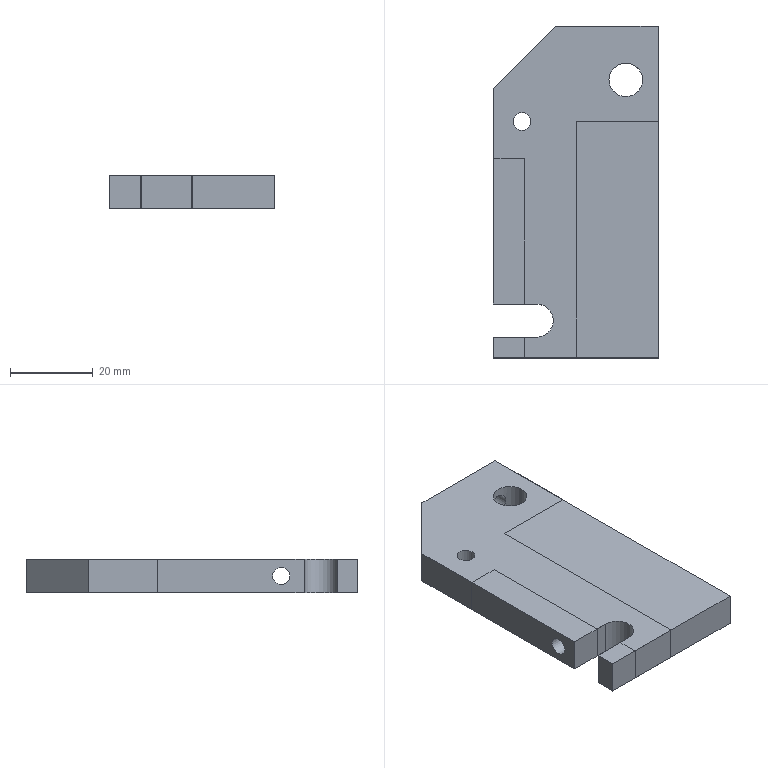NC program | NX | posted with a generic post | part box 40 x 80 x 8 mm
Whole program:
N10 G17 G21 G94 G90
(ADAPTIVE_MILLING , TOOL : D10-30-D10-75-3T-ROUGH)
N12 T01 M6
N14 G54
N16 G17 G0 G90 X-0.719 Y33.082 S3000 M3
N18 G43 Z20. H1
N20 Z3.1
N22 G94 G1 X-0.716 Y32.932 Z2.163 F1500.
N24 X-0.713 Y32.782 Z1.792
N26 X-0.71 Y32.632 Z1.52
N28 X-0.707 Y32.482 Z1.3
N30 X-0.704 Y32.332 Z1.116
N32 X-0.701 Y32.182 Z0.958
N34 X-0.698 Y32.032 Z0.82
N36 X-0.695 Y31.882 Z0.7
N38 X-0.692 Y31.732 Z0.595
N40 X-0.688 Y31.582 Z0.502
N42 X-0.685 Y31.432 Z0.421
N44 X-0.682 Y31.282 Z0.35
N46 X-0.679 Y31.132 Z0.29
N48 X-0.676 Y30.982 Z0.238
N50 X-0.673 Y30.832 Z0.195
N52 X-0.67 Y30.682 Z0.161
N54 X-0.667 Y30.532 Z0.134
N56 X-0.664 Y30.382 Z0.115
N58 X-0.661 Y30.232 Z0.104
N60 X-0.658 Y30.082 Z0.1
N62 X-0.624 Y28.462
N64 G3 X0.024 Y27.54 R1.011
N66 X2.218 Y27.216 R8.479
N68 X11.422 Y27.1 R194.322
N70 G1 X39.422 Y27.099
N72 G2 X44.024 Y24.676 R5.712
N74 X45.709 Y20.39 R9.765
N76 X46.075 Y14.707 R38.659
N78 G1 X46.098 Y7.207
N80 X46.096 Y-20.46
N82 G2 X43.644 Y-25.047 R5.72
N84 X39.252 Y-26.733 R9.919
N86 X33.467 Y-27.079 R41.286
N88 G1 X26.218 Y-27.1
N90 X-39.462 Y-27.097
N92 G2 X-44.048 Y-24.645 R5.719
N94 X-45.734 Y-20.252 R9.931
N96 X-46.08 Y-14.467 R41.275
N98 G1 X-46.101 Y-7.217
N100 X-46.099 Y20.46
N102 G2 X-43.646 Y25.047 R5.719
N104 X-39.253 Y26.732 R9.931
N106 X-33.469 Y27.079 R41.275
N108 G1 X-26.219 Y27.1
N110 X-2.119 Y27.097
N112 G2 X2.81 Y26.809 R819.319
N114 G3 X12.522 Y26.701 R286.424
N116 G1 X37.722 Y26.699
N118 G2 X43.64 Y23.314 R7.101
N120 X45.299 Y18.58 R11.962
N122 X45.672 Y12.446 R45.859
N124 G1 X45.698 Y4.546
N126 X45.697 Y-18.722
N128 G2 X42.35 Y-24.615 R7.089
N130 X37.576 Y-26.3 R11.916
N132 X31.642 Y-26.671 R44.728
N134 G1 X23.692 Y-26.699
N136 X-37.723 Y-26.698
N138 G2 X-43.617 Y-23.349 R7.088
N140 X-45.301 Y-18.575 R11.921
N142 X-45.678 Y-12.191 R47.36
N144 G1 X-45.7 Y-5.941
N146 Y18.622
N148 G2 X-42.35 Y24.616 R7.087
N150 X-37.576 Y26.3 R11.921
N152 X-31.193 Y26.677 R47.36
N154 G1 X-24.943 Y26.699
N156 X-3.73 Y26.698
N158 G2 X2.84 Y26.421 R237.984
N160 G3 X13.622 Y26.301 R334.657
N162 G1 X35.972 Y26.3
N164 G2 X43.459 Y21.85 R8.144
N166 X44.965 Y16.642 R14.601
N168 X45.282 Y9.653 R64.652
N170 G1 X45.298 Y3.003
N172 X45.297 Y-17.047
N174 G2 X40.938 Y-24.409 R8.12
N176 X35.89 Y-25.934 R14.195
N178 X29.303 Y-26.277 R56.959
N180 G1 X21.453 Y-26.299
N182 X-36.047 Y-26.298
N184 G2 X-43.413 Y-21.934 R8.118
N186 X-44.935 Y-16.889 R14.217
N188 X-45.279 Y-10.252 R57.3
N190 G1 X-45.3 Y-2.552
N192 X-45.299 Y17.048
N194 G2 X-40.936 Y24.412 R8.118
N196 X-35.89 Y25.934 R14.218
N198 X-29.253 Y26.277 R57.3
N200 G1 X-21.553 Y26.299
N202 X-4.979 Y26.298
N204 G2 X2.923 Y26.026 R253.671
N206 G3 X15.222 Y25.901 R401.917
N208 G1 X34.472 Y25.9
N210 G2 X38.99 Y24.999 R9.989
N212 X43.369 Y20.219 R9.282
N214 X44.633 Y14.737 R18.014
N216 X44.889 Y6.893 R93.499
N218 G1 X44.897 Y1.943
N220 Y-15.472
N222 G2 X43.996 Y-19.99 R9.988
N224 X39.156 Y-24.396 R9.305
N226 X33.568 Y-25.65 R18.418
N228 X25.924 Y-25.89 R96.511
N230 G1 X20.974 Y-25.899
N232 X-34.473 Y-25.898
N234 G2 X-38.991 Y-24.997 R9.99
N236 X-43.369 Y-20.219 R9.282
N238 X-44.635 Y-14.737 R18.005
N240 X-44.891 Y-6.994 R92.212
N242 G1 X-44.9 Y-0.944
N244 X-44.899 Y15.472
N246 G2 X-43.998 Y19.99 R9.989
N248 X-39.221 Y24.368 R9.282
N250 X-33.738 Y25.634 R18.005
N252 X-25.995 Y25.89 R92.222
N254 G1 X-19.945 Y25.899
N256 X-6.179 Y25.898
N258 G2 X3.109 Y25.627 R288.66
N260 G3 X15.272 Y25.501 R440.021
N262 G1 X33.222 Y25.499
N264 G2 X37.685 Y24.777 R11.809
N266 X42.744 Y19.814 R9.555
N268 X44.158 Y14.317 R17.56
N270 X44.48 Y6.828 R75.391
N272 G1 X44.497 Y-0.372
N274 X44.496 Y-14.122
N276 G2 X43.864 Y-18.451 R12.256
N278 X38.889 Y-23.708 R9.502
N280 X33.202 Y-25.171 R17.61
N282 X25.462 Y-25.484 R79.927
N284 G1 X18.862 Y-25.498
N286 X-33.123
N288 G2 X-37.453 Y-24.865 R12.256
N290 X-42.708 Y-19.891 R9.504
N292 X-44.161 Y-14.304 R17.449
N294 X-44.484 Y-6.614 R76.99
N296 G1 X-44.499 Y-0.564
N298 Y14.122
N300 G2 X-43.866 Y18.452 R12.255
N302 X-38.892 Y23.707 R9.504
N304 X-33.305 Y25.16 R17.45
N306 X-25.615 Y25.483 R76.991
N308 G1 X-19.565 Y25.498
N310 X-7.279
N312 G2 X3.101 Y25.232 R315.659
N314 G3 X15.572 Y25.102 R473.15
N316 G1 X31.922 Y25.1
N318 G2 X36.321 Y24.557 R14.429
N320 X42.155 Y19.383 R9.828
N322 X43.719 Y13.621 R17.669
N324 X44.08 Y5.583 R75.857
N326 G1 X44.097 Y-2.117
N328 G2 X44.075 Y-14.022 R854.441
N330 X42.651 Y-19.324 R10.75
N332 X37.33 Y-23.618 R10.507
N334 X31.526 Y-24.834 R21.057
N336 X23.432 Y-25.088 R104.823
N338 G1 X16.832 Y-25.098
N340 X-31.873 Y-25.097
N342 G2 X-36.178 Y-24.598 R14.783
N344 X-42.154 Y-19.384 R9.816
N346 X-43.702 Y-13.771 R17.466
N348 X-44.079 Y-5.985 R70.636
N350 G1 X-44.099 Y0.665
N352 G2 X-44.077 Y14.021 R944.397
N354 X-42.652 Y19.326 R10.747
N356 X-37.473 Y23.562 R10.454
N358 X-31.828 Y24.805 R20.302
N360 X-23.286 Y25.089 R100.222
N362 G1 X-18.336 Y25.098
N364 G2 X-3.43 Y25.04 R736.675
N366 G3 X16.822 Y24.702 R491.196
N368 G1 X30.672 Y24.7
N370 G2 X35.088 Y24.271 R17.569
N372 X41.664 Y18.796 R10.156
N374 X43.286 Y12.942 R18.042
N376 X43.67 Y5.356 R69.858
N378 G1 X43.696 Y-1.794
N380 G2 X43.664 Y-13.221 R565.835
N382 X42.301 Y-18.495 R11.448
N384 X36.974 Y-23.04 R10.705
N386 X31.047 Y-24.387 R20.607
N388 X22.655 Y-24.686 R96.522
N390 G1 X16.055 Y-24.698
N392 X-30.673 Y-24.697
N394 G2 X-35.138 Y-24.256 R17.414
N396 X-41.664 Y-18.798 R10.155
N398 X-43.287 Y-12.943 R18.041
N400 X-43.673 Y-5.307 R69.917
N402 G1 X-43.699 Y1.843
N404 G2 X-43.667 Y13.221 R562.693
N406 X-42.229 Y18.624 R11.384
N408 X-36.884 Y23.077 R10.77
N410 X-31.05 Y24.386 R20.792
N412 X-22.658 Y24.686 R96.37
N414 G1 X-17.158 Y24.698
N416 G2 X-2.78 Y24.616 R565.256
N418 G3 X17.222 Y24.302 R497.288
N420 G1 X29.422 Y24.301
N422 G2 X33.949 Y23.949 R21.442
N424 X41.202 Y18.191 R10.484
N426 X42.861 Y12.245 R18.494
N428 X43.267 Y4.51 R69.668
N430 X43.271 Y-12.072 R903.237
N432 X42.184 Y-17.22 R12.904
N434 X36.655 Y-22.454 R10.785
N436 X30.707 Y-23.927 R20.022
N438 X22.318 Y-24.28 R85.309
N440 G1 X14.618 Y-24.298
N442 X-29.473 Y-24.297
N444 G2 X-34.048 Y-23.924 R20.815
N446 X-41.198 Y-18.199 R10.48
N448 X-42.856 Y-12.295 R18.441
N450 X-43.27 Y-4.46 R69.348
N452 X-43.273 Y12.072 R903.184
N454 X-42.187 Y17.22 R12.901
N456 X-36.649 Y22.457 R10.788
N458 X-30.651 Y23.933 R20.145
N460 X-22.311 Y24.28 R86.022
N462 X-3.762 Y24.234 R842.135
N464 G3 X16.972 Y23.902 R589.615
N466 G2 X30.272 Y23.87 R817.304
N468 X35.433 Y22.825 R13.687
N470 X40.947 Y17.183 R11.01
N472 X42.497 Y11.103 R20.146
N474 X42.877 Y2.565 R83.861
N476 X42.865 Y-11.271 R673.681
N478 X41.821 Y-16.433 R13.68
N480 X36.181 Y-21.947 R11.008
N482 X30.101 Y-23.498 R20.156
N484 X22.063 Y-23.873 R79.7
N486 G1 X13.763 Y-23.897
N488 X-28.273
N490 G2 X-33.005 Y-23.579 R24.995
N492 X-40.778 Y-17.537 R10.798
N494 X-42.444 Y-11.542 R19.054
N496 X-42.872 Y-3.308 R72.694
N498 X-42.868 Y11.272 R673.669
N500 X-41.823 Y16.433 R13.677
N502 X-36.131 Y21.969 R11.023
N504 X-30.047 Y23.504 R20.331
N506 X-21.759 Y23.876 R82.622
N508 X-2.86 Y23.807 R680.934
N510 G3 X18.222 Y23.502 R579.313
N512 G2 X29.521 Y23.465 R553.103
N514 X34.784 Y22.41 R14.313
N516 X40.507 Y16.586 R11.272
N518 X42.077 Y10.458 R20.555
N520 X42.469 Y2.372 R79.047
N522 X42.459 Y-10.528 R490.91
N524 X41.424 Y-15.744 R14.313
N526 X35.702 Y-21.453 R11.233
N528 X29.635 Y-23.057 R20.14
N530 X21.15 Y-23.472 R78.544
N532 G1 X12.9 Y-23.497
N534 X-27.223
N536 G2 X-32.059 Y-23.212 R28.734
N538 X-40.389 Y-16.838 R11.113
N540 X-42.057 Y-10.635 R19.958
N542 X-42.468 Y-2.599 R75.097
N544 X-42.466 Y10.422 R554.767
N546 X-41.505 Y15.554 R14.678
N548 X-35.704 Y21.452 R11.207
N550 X-29.438 Y23.08 R20.455
N552 X-21.051 Y23.473 R81.406
N554 X4.464 Y23.214 R604.269
N556 G3 X25.422 Y23.102 R966.669
N558 G2 X30.615 Y22.917 R44.386
N560 X37.603 Y19.646 R11.532
N562 X40.882 Y13.796 R13.568
N564 X41.902 Y7.037 R30.903
N566 X42.094 Y-4.26 R214.857
N568 X42.002 Y-10.708 R100.555
N570 X40.299 Y-16.505 R12.789
N572 X34.425 Y-21.32 R11.94
N574 X28.049 Y-22.746 R23.095
N576 X19.108 Y-23.081 R101.832
N578 G1 X11.959 Y-23.097
N580 X-26.673 Y-23.095
N582 G2 X-31.703 Y-22.741 R26.76
N584 X-39.936 Y-16.294 R11.35
N586 X-41.634 Y-10.045 R20.219
N588 X-42.068 Y-1.711 R75.709
N590 X-42.05 Y9.939 R336.332
N592 X-40.915 Y15.336 R14.486
N594 X-35.093 Y21.03 R11.506
N596 X-28.874 Y22.654 R20.788
N598 X-20.638 Y23.067 R78.035
N600 X4.214 Y22.821 R594.688
N602 G3 X25.422 Y22.701 R984.655
N604 G2 X30.559 Y22.421 R33.455
N606 X39.529 Y15.671 R11.636
N608 X41.223 Y9.372 R20.737
N610 X41.664 Y0.887 R77.377
N612 X41.644 Y-9.212 R261.519
N614 X40.525 Y-14.666 R15.127
N616 X34.54 Y-20.59 R11.713
N618 X28.127 Y-22.254 R21.272
N620 X19.542 Y-22.669 R82.502
N622 G1 X11.792 Y-22.696
N624 X-25.523
N626 G2 X-30.757 Y-22.384 R31.453
N628 X-39.528 Y-15.672 R11.618
N630 X-41.224 Y-9.374 R20.756
N632 X-41.668 Y-0.739 R78.339
N634 X-41.644 Y9.26 R252.258
N636 X-40.528 Y14.664 R15.037
N638 X-34.536 Y20.591 R11.713
N640 X-28.169 Y22.248 R21.245
N642 X-19.383 Y22.671 R83.267
N644 X3.964 Y22.428 R587.164
N646 G3 X25.172 Y22.298 R993.4
N648 G2 X30.45 Y21.916 R28.573
N650 X39.063 Y15.188 R11.812
N652 X40.81 Y8.749 R21.011
N654 X41.264 Y0.016 R79.088
N656 X41.233 Y-8.633 R189.322
N658 X40.065 Y-14.178 R15.34
N660 X33.936 Y-20.181 R11.943
N662 X27.52 Y-21.839 R21.672
N664 X18.735 Y-22.269 R83.286
N666 G1 X9.935 Y-22.296
N668 X-24.573 Y-22.295
N670 G2 X-29.959 Y-22. R34.738
N672 X-39.095 Y-15.122 R11.851
N674 X-40.814 Y-8.726 R21.164
N676 X-41.263 Y-0.292 R77.052
N678 X-41.231 Y8.707 R186.101
N680 X-40.035 Y14.249 R15.159
N682 X-33.986 Y20.157 R11.94
N684 X-27.622 Y21.826 R21.522
N686 X-18.988 Y22.266 R80.32
N688 X3.416 Y22.041 R556.79
N690 G3 X24.422 Y21.898 R946.655
N692 G2 X29.702 Y21.531 R30.293
N694 X38.634 Y14.644 R12.023
N696 X40.369 Y8.355 R21.059
N698 X40.852 Y0.024 R72.506
N700 X40.81 Y-8.274 R136.124
N702 X39.518 Y-13.892 R15.097
N704 X33.372 Y-19.76 R12.174
N706 X26.908 Y-21.427 R22.054
N708 X18.473 Y-21.861 R80.674
N710 G1 X9.073 Y-21.896
N712 X-23.573 Y-21.895
N714 G2 X-29.012 Y-21.64 R40.091
N716 X-36.049 Y-18.319 R12.222
N718 X-39.538 Y-12.298 R14.066
N720 X-40.667 Y-5.303 R31.062
N722 X-40.823 Y8.092 R160.177
N724 X-39.617 Y13.68 R15.53
N726 X-33.449 Y19.724 R12.121
N728 X-27.042 Y21.41 R21.8
N730 X-18.209 Y21.865 R81.15
N732 X4.227 Y21.625 R606.053
N734 G3 X23.972 Y21.495 R949.588
N736 G2 X29.396 Y21.064 R28.549
N738 X38.163 Y14.199 R12.184
N740 X39.949 Y7.821 R21.194
N742 X40.446 Y-0.409 R71.049
N744 X40.391 Y-7.807 R102.754
N746 X38.996 Y-13.551 R15.059
N748 X32.883 Y-19.311 R12.36
N750 X26.275 Y-21.021 R22.401
N752 X17.691 Y-21.461 R82.28
N754 G1 X8.291 Y-21.496
N756 X-22.659 Y-21.495
N758 G2 X-28.349 Y-21.239 R43.043
N760 X-35.311 Y-18.105 R12.542
N762 X-39.015 Y-12.066 R13.938
N764 X-40.228 Y-5.138 R29.621
N766 X-40.41 Y7.555 R130.078
N768 X-39.15 Y13.233 R15.667
N770 X-32.885 Y19.309 R12.324
N772 X-26.279 Y21.019 R22.415
N774 X-17.295 Y21.466 R84.914
N776 X3.213 Y21.247 R558.526
N778 G3 X23.473 Y21.092 R982.573
N780 G2 X28.944 Y20.626 R27.902
N782 X37.781 Y13.578 R12.376
N784 X39.557 Y7.094 R21.817
N786 X40.053 Y-1.637 R76.269
N788 X39.911 Y-8.032 R59.227
N790 X37.852 Y-14.287 R13.739
N792 X31.789 Y-19.13 R12.961
N794 X25.186 Y-20.669 R24.327
N796 X16.049 Y-21.07 R96.113
N798 G1 X7.249 Y-21.095
N800 X-21.801
N802 G2 X-27.592 Y-20.852 R46.657
N804 X-34.274 Y-18.134 R13.003
N806 X-38.408 Y-12.066 R13.591
N808 X-39.76 Y-5.268 R27.304
N810 X-40.001 Y6.923 R109.018
N812 X-38.747 Y12.654 R16.047
N814 X-32.387 Y18.869 R12.481
N816 X-25.737 Y20.603 R22.617
N818 X-16.903 Y21.061 R82.904
N820 X3.857 Y20.835 R587.071
N822 G3 X22.824 Y20.691 R971.585
N824 G2 X28.394 Y20.211 R28.452
N826 X37.342 Y13.087 R12.536
N828 X39.15 Y6.5 R22.085
N830 X39.65 Y-2.481 R76.95
N832 X39.376 Y-8.418 R38.219
N834 X35.884 Y-15.687 R12.754
N836 X29.751 Y-19.248 R14.592
N838 X22.713 Y-20.43 R31.386
N840 X11.869 Y-20.689 R169.176
N842 G1 X6.369 Y-20.695
N844 X-21.481 Y-20.693
N846 G2 X-27.22 Y-20.414 R42.746
N848 X-34.142 Y-17.395 R13.009
N850 X-38.118 Y-11.155 R14.099
N852 X-39.382 Y-4.338 R29.122
N854 X-39.579 Y6.504 R90.847
N856 X-38.237 Y12.317 R15.896
N858 X-31.834 Y18.459 R12.668
N860 X-25.229 Y20.185 R22.836
N862 X-16.496 Y20.655 R80.678
N864 X4.153 Y20.431 R597.167
N866 G3 X22.026 Y20.292 R917.556
N868 G2 X27.698 Y19.83 R30.306
N870 X36.943 Y12.521 R12.715
N872 X38.759 Y5.788 R22.609
N874 X39.14 Y-6.242 R72.388
N876 X37.59 Y-12.252 R15.394
N878 X31.199 Y-18.09 R12.902
N880 X24.534 Y-19.792 R23.424
N882 X15.55 Y-20.259 R84.976
N884 G1 X5.651 Y-20.295
N886 X-20.099 Y-20.294
N888 G2 X-26.192 Y-20.066 R53.835
N890 X-32.664 Y-17.74 R13.856
N892 X-37.344 Y-11.597 R13.443
N894 X-38.873 Y-4.833 R25.548
N896 X-39.141 Y6.253 R73.358
N898 X-37.608 Y12.22 R15.402
N900 X-31.255 Y18.065 R12.886
N902 X-24.645 Y19.778 R23.234
N904 X-15.513 Y20.257 R83.462
N906 X3.407 Y20.046 R571.534
N908 G3 X21.627 Y19.888 R982.087
N910 G2 X27.296 Y19.389 R29.352
N912 X36.49 Y12.08 R12.846
N914 X38.341 Y5.303 R22.69
N916 X38.711 Y-5.826 R62.165
N918 X37.006 Y-12.047 R15.207
N920 X30.672 Y-17.676 R13.094
N922 X23.96 Y-19.385 R23.746
N924 X14.677 Y-19.86 R87.473
N926 G1 X4.777 Y-19.894
N928 X-19.823 Y-19.893
N930 G2 X-26.012 Y-19.608 R47.304
N932 X-32.784 Y-16.854 R13.577
N934 X-37.133 Y-10.534 R14.038
N936 X-38.528 Y-3.642 R27.978
N938 X-38.723 Y5.697 R63.623
N940 X-37.115 Y11.848 R15.459
N942 X-30.696 Y17.664 R13.055
N944 X-23.938 Y19.387 R23.763
N946 X-14.605 Y19.858 R86.849
N948 X4.251 Y19.63 R626.009
N950 G3 X20.629 Y19.492 R875.153
N952 G2 X26.454 Y19.041 R32.844
N954 X36.072 Y11.572 R13.007
N956 X37.919 Y4.845 R22.834
N958 X38.272 Y-5.483 R53.279
N960 X36.45 Y-11.783 R14.988
N962 X30.058 Y-17.303 R13.289
N964 X23.24 Y-18.997 R24.401
N966 X14.256 Y-19.456 R88.108
N968 X3.756 Y-19.494 R739.957
N970 G1 X-19.044 Y-19.493
N972 G2 X-25.334 Y-19.218 R50.202
N974 X-31.905 Y-16.73 R14.003
N976 X-36.564 Y-10.423 R13.855
N978 X-38.094 Y-3.357 R26.939
N980 X-38.261 Y5.63 R51.941
N982 X-36.32 Y12.005 R14.723
N984 X-29.918 Y17.362 R13.387
N986 X-23.138 Y19.009 R24.81
N988 X-13.553 Y19.458 R92.085
N990 X4.249 Y19.231 R654.526
N992 G3 X20.082 Y19.091 R885.67
N994 G2 X25.956 Y18.625 R32.98
N996 X35.62 Y11.142 R13.126
N998 X37.488 Y4.469 R22.737
N1000 X37.818 Y-5.257 R45.53
N1002 X35.701 Y-11.824 R14.535
N1004 X29.308 Y-16.989 R13.613
N1006 X22.419 Y-18.622 R25.473
N1008 X12.933 Y-19.063 R96.892
N1010 G1 X3.033 Y-19.094
N1012 X-18.267 Y-19.093
N1014 G2 X-24.509 Y-18.846 R55.144
N1016 X-31.021 Y-16.586 R14.584
N1018 X-36.019 Y-10.24 R13.736
N1020 X-37.646 Y-3.196 R25.956
N1022 X-37.812 Y5.339 R44.396
N1024 X-35.637 Y11.923 R14.417
N1026 X-29.299 Y16.992 R13.641
N1028 X-22.362 Y18.627 R25.593
N1030 X-12.625 Y19.055 R96.329
N1032 X5.64 Y18.808 R830.443
N1034 G3 X19.835 Y18.686 R992.222
N1036 G2 X25.751 Y18.15 R30.641
N1038 X35.249 Y10.55 R13.258
N1040 X37.115 Y3.676 R23.421
N1042 X37.364 Y-4.953 R39.363
N1044 X35.065 Y-11.654 R14.294
N1046 X28.741 Y-16.599 R13.827
N1048 X21.801 Y-18.223 R25.939
N1050 X12.215 Y-18.664 R99.214
N1052 G1 X2.315 Y-18.693
N1054 X-17.485 Y-18.692
N1056 G2 X-23.976 Y-18.438 R57.076
N1058 X-30.502 Y-16.189 R14.792
N1060 X-35.607 Y-9.727 R13.853
N1062 X-37.245 Y-2.585 R26.233
N1064 X-37.35 Y5.101 R37.728
N1066 X-34.869 Y11.935 R14.079
N1068 X-28.558 Y16.672 R13.984
N1070 X-21.402 Y18.265 R26.945
N1072 X-11.113 Y18.653 R106.722
N1074 X5.69 Y18.409 R932.667
N1076 G3 X19.188 Y18.287 R962.997
N1078 G2 X25.106 Y17.768 R31.891
N1080 X34.77 Y10.189 R13.362
N1082 X36.687 Y3.279 R23.172
N1084 X36.881 Y-4.849 R33.716
N1086 X33.961 Y-12.083 R13.771
N1088 X27.474 Y-16.478 R14.551
N1090 X20.435 Y-17.902 R29.004
N1092 X10.045 Y-18.276 R124.533
N1094 G1 X1.795 Y-18.293
N1096 X-16.705 Y-18.292
N1098 G2 X-23.297 Y-18.049 R60.912
N1100 X-29.724 Y-15.961 R15.248
N1102 X-35.141 Y-9.355 R13.853
N1104 X-36.816 Y-2.222 R25.795
N1106 X-36.829 Y5.261 R31.386
N1108 X-33.148 Y12.984 R13.375
N1110 X-26.692 Y16.738 R15.409
N1112 X-19.412 Y17.988 R32.839
N1114 X-7.318 Y18.23 R150.887
N1116 G1 X5.292 Y18.016
N1118 G3 X18.541 Y17.888 R935.596
N1120 G2 X24.608 Y17.356 R32.531
N1122 X34.393 Y9.619 R13.493
N1124 X36.308 Y2.499 R23.601
N1126 X36.36 Y-4.929 R28.391
N1128 X28.757 Y-15.318 R13.27
N1130 X21.904 Y-17.261 R23.118
N1132 X13.128 Y-17.83 R74.415
N1134 X1.028 Y-17.893 R743.615
N1136 G1 X-16.022 Y-17.892
N1138 G2 X-22.714 Y-17.649 R62.897
N1140 X-29.191 Y-15.576 R15.52
N1142 X-34.647 Y-9.051 R13.878
N1144 X-36.4 Y-1.686 R25.354
N1146 X-36.296 Y5.343 R26.524
N1148 X-28.806 Y15.294 R13.239
N1150 X-21.906 Y17.26 R23.071
N1152 X-13.029 Y17.817 R72.463
N1154 X2.704 Y17.662 R497.207
N1156 G3 X17.844 Y17.491 R903.429
N1158 G2 X24.013 Y16.967 R33.955
N1160 X33.96 Y9.174 R13.605
N1162 X35.914 Y1.759 R23.555
N1164 X35.762 Y-5.313 R23.611
N1166 X28.501 Y-14.789 R13.214
N1168 X21.67 Y-16.812 R22.598
N1170 X12.747 Y-17.424 R71.359
N1172 X0.648 Y-17.493 R734.368
N1174 G1 X-15.302 Y-17.492
N1176 G2 X-22.045 Y-17.259 R66.65
N1178 X-28.456 Y-15.314 R16.004
N1180 X-34.163 Y-8.724 R13.882
N1182 X-35.989 Y-1.02 R24.816
N1184 X-35.671 Y5.746 R22.1
N1186 X-28.573 Y14.751 R13.184
N1188 X-21.652 Y16.813 R22.55
N1190 X-12.878 Y17.404 R68.442
N1192 X2.902 Y17.258 R480.313
N1194 G3 X17.198 Y17.094 R882.251
N1196 G2 X23.369 Y16.587 R35.421
N1198 X33.538 Y8.708 R13.743
N1200 X35.524 Y0.794 R23.308
N1202 X35.021 Y-6.051 R19.456
N1204 X28.152 Y-14.303 R13.184
N1206 X21.341 Y-16.376 R22.347
N1208 X12.571 Y-17.014 R68.364
N1210 X-0.279 Y-17.092 R730.792
N1212 G1 X-14.529 Y-17.091
N1214 G2 X-21.522 Y-16.855 R69.045
N1216 X-27.852 Y-14.972 R16.266
N1218 X-33.76 Y-8.217 R13.973
N1220 X-35.609 Y0.742 R24.549
N1222 X-34.525 Y7.506 R16.714
N1224 X-27.932 Y14.413 R13.31
N1226 X-20.942 Y16.434 R23.14
N1228 X-11.566 Y17.008 R73.414
N1230 X5.489 Y16.815 R674.704
N1232 G1 X17.251 Y16.683
N1234 G2 X23.263 Y16.099 R31.697
N1236 X33.129 Y8.22 R13.795
N1238 X34.926 Y-3.844 R22.417
N1240 X27.739 Y-13.852 R13.19
N1242 X20.883 Y-15.961 R22.337
N1244 X12.063 Y-16.611 R68.122
N1246 X-0.786 Y-16.692 R707.952
N1248 G1 X-14.386 Y-16.69
N1250 G2 X-21.277 Y-16.418 R61.816
N1252 X-27.751 Y-14.341 R15.925
N1254 X-33.387 Y-7.642 R14.15
N1256 X-34.937 Y3.78 R22.555
N1258 X-27.692 Y13.875 R13.202
N1260 X-20.832 Y15.967 R22.434
N1262 X-11.66 Y16.593 R67.553
N1264 X3.996 Y16.44 R526.605
N1266 G1 X16.054 Y16.298
N1268 G2 X22.227 Y15.803 R37.269
N1270 X29.919 Y11.842 R14.142
N1272 X33.727 Y5.045 R16.075
N1274 X34.385 Y-3.761 R20.368
N1276 X27.366 Y-13.379 R13.115
N1278 X20.524 Y-15.53 R22.115
N1280 X11.807 Y-16.203 R66.027
N1282 X-1.043 Y-16.292 R632.503
N1284 G1 X-13.193 Y-16.291
N1286 G2 X-20.386 Y-16.057 R73.446
N1288 X-26.827 Y-14.19 R16.768
N1290 X-32.908 Y-7.312 R14.091
N1292 X-34.418 Y3.555 R20.674
N1294 X-27.454 Y13.331 R13.103
N1296 X-20.617 Y15.512 R21.857
N1298 X-11.649 Y16.177 R63.279
N1300 X4.145 Y16.037 R495.174
N1302 G1 X15.958 Y15.891
N1304 G2 X22.122 Y15.32 R33.936
N1306 X32.4 Y7.051 R14.011
N1308 X33.874 Y-3.411 R18.985
N1310 X27.118 Y-12.837 R12.998
N1312 X20.261 Y-15.083 R21.628
N1314 X11.797 Y-15.786 R62.252
N1316 X-1.952 Y-15.891 R560.472
N1318 X-16.752 Y-15.845 R830.871
N1320 X-22.946 Y-15.114 R27.937
N1322 X-32.306 Y-7.253 R13.905
N1324 X-33.887 Y3.335 R19.013
N1326 X-27.054 Y12.872 R13.012
N1328 X-20.133 Y15.101 R21.81
N1330 X-11.065 Y15.77 R63.427
N1332 X4.044 Y15.639 R489.063
N1334 G1 X15.411 Y15.493
N1336 G2 X21.625 Y14.916 R34.431
N1338 X32.061 Y6.396 R14.094
N1340 X33.319 Y-3.25 R17.46
N1342 X26.941 Y-12.249 R12.834
N1344 X20.32 Y-14.576 R20.701
N1346 X12.164 Y-15.355 R55.453
N1348 X-3.234 Y-15.491 R491.172
N1350 X-16.384 Y-15.438 R624.393
N1352 X-22.573 Y-14.677 R27.426
N1354 X-31.975 Y-6.588 R13.987
N1356 X-33.331 Y3.184 R17.5
N1358 X-26.813 Y12.321 R12.859
N1360 X-20.025 Y14.625 R21.097
N1362 X-11.563 Y15.341 R57.111
N1364 X3.495 Y15.248 R397.416
N1366 G1 X14.614 Y15.102
N1368 G2 X20.932 Y14.554 R36.906
N1370 X28.694 Y10.462 R14.357
N1372 X32.803 Y1.744 R15.97
N1374 X31.676 Y-6.352 R13.742
N1376 X25.611 Y-12.294 R13.263
N1378 X18.735 Y-14.356 R23.017
N1380 X10.015 Y-15.002 R69.474
N1382 X-2.835 Y-15.091 R652.122
N1384 X-15.834 Y-15.037 R611.189
N1386 X-22.074 Y-14.275 R27.815
N1388 X-31.633 Y-5.929 R14.028
N1390 X-32.731 Y3.176 R16.049
N1392 X-26.508 Y11.802 R12.7
N1394 X-19.791 Y14.168 R20.637
N1396 X-11.533 Y14.92 R53.93
N1398 X0.016 Y14.905 R280.539
N1400 G1 X13.917 Y14.709
N1402 G2 X20.336 Y14.172 R38.57
N1404 X27.785 Y10.504 R14.595
N1406 X32.201 Y-2.704 R15.164
N1408 X26.326 Y-11.203 R12.474
N1410 X19.564 Y-13.715 R20.054
N1412 X11.063 Y-14.553 R54.68
N1414 X-2.786 Y-14.69 R440.118
N1416 X-15.285 Y-14.636 R548.677
N1418 X-21.575 Y-13.873 R28.247
N1420 X-31.408 Y-4.929 R14.066
N1422 X-31.98 Y3.718 R14.489
N1424 X-26.071 Y11.356 R12.582
N1426 X-19.318 Y13.756 R20.513
N1428 X-10.611 Y14.523 R55.308
N1430 X0.488 Y14.496 R303.272
N1432 G1 X13.469 Y14.311
N1434 G2 X19.79 Y13.78 R38.997
N1436 X27.224 Y10.194 R14.737
N1438 X31.651 Y-2.215 R14.326
N1440 X25.971 Y-10.701 R12.253
N1442 X19.229 Y-13.276 R19.721
N1444 X10.783 Y-14.142 R52.98
N1446 X-4.116 Y-14.29 R442.474
N1448 X-15.415 Y-14.211 R347.123
N1450 X-21.683 Y-13.302 R25.385
N1452 X-31.293 Y-3.386 R14.012
N1454 X-30.669 Y5.455 R12.81
N1456 X-24.813 Y11.37 R12.952
N1458 X-18.06 Y13.481 R22.223
N1460 X-9.091 Y14.135 R63.193
N1462 X5.884 Y14.012 R534.292
N1464 X15.171 Y13.834 R309.842
N1466 X21.474 Y12.833 R24.759
N1468 X31.12 Y-1.345 R13.664
N1470 X25.916 Y-9.987 R11.909
N1472 X19.384 Y-12.727 R18.573
N1474 X11.602 Y-13.68 R45.614
N1476 X-1.045 Y-13.887 R273.472
N1478 X-14.395 Y-13.828 R542.747
N1480 X-20.635 Y-13.058 R28.397
N1482 X-31.173 Y0.444 R13.784
N1484 X-26.041 Y9.896 R11.847
N1486 X-19.547 Y12.68 R18.241
N1488 X-11.666 Y13.635 R43.467
N1490 X1.132 Y13.683 R226.996
N1492 X13.924 Y13.471 R917.871
N1494 X20.306 Y12.636 R28.559
N1496 X29.212 Y5.489 R13.733
N1498 X29.864 Y-3.888 R11.954
N1500 X24.464 Y-10.18 R12.232
N1502 X17.754 Y-12.556 R20.559
N1504 X9.2 Y-13.358 R57.49
N1506 X-5.149 Y-13.489 R481.019
N1508 X-14.947 Y-13.381 R216.144
N1510 X-21.24 Y-12.331 R23.635
N1512 X-30.451 Y-1.329 R13.361
N1514 X-25.888 Y9.214 R11.47
N1516 X-19.573 Y12.141 R17.339
N1518 X-11.607 Y13.205 R40.397
N1520 X-0.01 Y13.297 R191.75
N1522 X13.427 Y13.074 R891.122
N1524 X19.809 Y12.239 R28.877
N1526 X27.822 Y6.655 R13.731
N1528 X29.555 Y-2.513 R11.588
N1530 X24.58 Y-9.366 R11.638
N1532 X18.059 Y-11.985 R18.881
N1534 X10.07 Y-12.9 R48.362
N1536 X-2.927 Y-13.087 R312.547
N1538 X-13.776 Y-13.01 R327.426
N1540 X-20.148 Y-12.121 R26.652
N1542 X-28.35 Y-5.774 R13.501
N1544 X-29.081 Y3.972 R11.301
N1546 X-23.854 Y9.816 R12.101
N1548 X-17.224 Y12.138 R20.389
N1550 X-8.615 Y12.887 R55.083
N1552 X1.935 Y12.869 R309.572
N1554 X13.279 Y12.661 R497.853
N1556 X19.649 Y11.75 R27.338
N1558 X27.168 Y6.492 R13.493
N1560 X28.642 Y-3.091 R10.863
N1562 X23.755 Y-9.144 R11.616
N1564 X17.206 Y-11.652 R19.306
N1566 X8.861 Y-12.529 R52.142
N1568 X-5.987 Y-12.689 R415.971
N1570 X-14.684 Y-12.532 R136.47
N1572 X-21.033 Y-11.257 R21.451
N1574 X-28.286 Y-4.439 R12.799
N1576 X-25.575 Y7.743 R10.636
N1578 X-19.462 Y11.067 R15.647
N1580 X-12.029 Y12.301 R34.107
N1582 X-0.434 Y12.496 R148.171
N1584 X12.73 Y12.267 R564.571
N1586 X19.055 Y11.384 R28.061
N1588 X26.017 Y6.963 R13.503
N1590 X28.12 Y-2.241 R10.404
N1592 X23.565 Y-8.491 R11.121
N1594 X17.21 Y-11.132 R18.16
N1596 X9.227 Y-12.087 R46.536
N1598 X-4.87 Y-12.287 R321.241
N1600 X-13.968 Y-12.145 R155.837
N1602 X-20.286 Y-10.958 R22.347
N1604 X-27.023 Y-5.483 R12.698
N1606 X-25.291 Y7.054 R10.204
N1608 X-19.378 Y10.517 R14.869
N1610 X-12.066 Y11.851 R31.619
N1612 X-1.223 Y12.099 R127.626
N1614 X12.331 Y11.866 R495.871
N1616 X18.749 Y10.936 R27.6
N1618 X25.3 Y6.814 R13.217
N1620 X27.03 Y-3.094 R9.803
N1622 X22.185 Y-8.605 R11.354
N1624 X15.862 Y-10.902 R19.583
N1626 X7.861 Y-11.724 R52.86
N1628 X-12.086 Y-11.813 R395.256
N1630 X-18.468 Y-10.984 R28.398
N1632 X-24.98 Y-7.164 R13.4
N1634 X-27.453 Y1.702 R9.911
N1636 X-23.177 Y7.939 R10.691
N1638 X-17.005 Y10.627 R17.239
N1640 X-9.276 Y11.585 R41.822
N1642 X3.372 Y11.646 R227.4
N1644 X12.868 Y11.409 R198.83
N1646 X19.19 Y10.239 R23.395
N1648 X25.018 Y6.086 R12.298
N1650 X24.65 Y-5.585 R9.329
N1652 X19.199 Y-9.382 R13.303
N1654 X12.147 Y-10.98 R27.373
N1656 X1.962 Y-11.451 R107.713
N1658 X-11.537 Y-11.414 R374.544
N1660 X-17.873 Y-10.614 R29.059
N1662 X-24.099 Y-7.147 R13.281
N1664 X-26.599 Y1.806 R9.393
N1666 X-22.264 Y7.75 R10.545
N1668 X-16.104 Y10.302 R17.521
N1670 X-8.316 Y11.195 R43.848
N1672 X3.933 Y11.237 R244.114
N1674 X12.578 Y10.998 R159.593
N1676 X18.842 Y9.793 R22.844
N1678 X24.275 Y5.913 R11.746
N1680 X24.17 Y-4.93 R8.905
N1682 X18.793 Y-8.903 R12.686
N1684 X12.055 Y-10.525 R25.768
N1686 X2.623 Y-11.034 R93.275
N1688 X-11.126 Y-11.009 R338.655
N1690 X-17.508 Y-10.182 R28.621
N1692 X-23.366 Y-6.943 R12.851
N1694 X-24.038 Y5.085 R8.924
N1696 X-18.666 Y8.934 R12.777
N1698 X-11.912 Y10.489 R25.775
N1700 X-2.325 Y10.882 R90.44
N1702 X11.173 Y10.66 R326.86
N1704 X17.387 Y9.72 R26.958
N1706 X22.747 Y6.621 R12.191
N1708 X23.491 Y-4.468 R8.53
N1710 X18.433 Y-8.389 R12.11
N1712 X11.765 Y-10.089 R24.323
N1714 X2.285 Y-10.63 R88.41
N1716 X-10.913 Y-10.597 R285.15
N1718 X-17.19 Y-9.736 R27.554
N1720 X-22.653 Y-6.688 R12.259
N1722 X-23.477 Y4.466 R8.508
N1724 X-18.28 Y8.431 R12.135
N1726 X-11.643 Y10.047 R24.336
N1728 X-2.058 Y10.473 R85.443
N1730 X10.59 Y10.269 R298.844
N1732 X16.808 Y9.349 R27.354
N1734 X21.861 Y6.512 R11.691
N1736 X22.862 Y-3.861 R8.138
N1738 X18.062 Y-7.856 R11.452
N1740 X11.674 Y-9.62 R22.456
N1742 X2.449 Y-10.217 R78.354
N1744 X-10.599 Y-10.187 R250.451
N1746 X-16.918 Y-9.274 R26.485
N1748 X-21.973 Y-6.362 R11.4
N1750 X-22.82 Y3.895 R8.115
N1752 X-17.868 Y7.917 R11.487
N1754 X-11.456 Y9.591 R22.712
N1756 X-2.774 Y10.058 R74.32
N1758 X10.223 Y9.867 R261.994
N1760 X16.388 Y8.93 R26.611
N1762 X21.15 Y6.18 R10.787
N1764 X22.119 Y-3.324 R7.769
N1766 X17.468 Y-7.405 R10.906
N1768 X11.144 Y-9.208 R21.458
N1770 X2.42 Y-9.805 R73.518
N1772 X-10.229 Y-9.78 R222.292
N1774 X-16.398 Y-8.88 R26.041
N1776 X-21.152 Y-6.136 R10.657
N1778 X-22.077 Y3.352 R7.742
N1780 X-17.395 Y7.406 R10.87
N1782 X-11.053 Y9.155 R21.319
N1784 X-2.273 Y9.648 R71.347
N1786 X10.074 Y9.451 R216.136
N1788 X16.031 Y8.486 R24.851
N1790 X20.452 Y5.767 R9.672
N1792 X21.215 Y-2.945 R7.438
N1794 X16.614 Y-7.057 R10.513
N1796 X10.483 Y-8.811 R20.856
N1798 X1.909 Y-9.403 R71.825
N1800 X-10.139 Y-9.358 R184.389
N1802 X-16.003 Y-8.444 R24.272
N1804 X-20.401 Y-5.774 R9.616
N1806 X-21.174 Y2.96 R7.408
N1808 X-16.56 Y7.042 R10.458
N1810 X-10.367 Y8.754 R20.696
N1812 X-1.686 Y9.239 R70.605
N1814 X9.76 Y9.043 R184.789
N1816 X15.373 Y8.13 R24.021
N1818 X19.585 Y5.461 R8.777
N1820 X20.262 Y-2.531 R7.129
N1822 X15.813 Y-6.657 R10.044
N1824 X10.037 Y-8.375 R19.644
N1826 X1.865 Y-8.989 R65.191
N1828 X-9.782 Y-8.948 R163.385
N1830 X-15.351 Y-8.08 R23.431
N1832 X-19.584 Y-5.396 R8.662
N1834 X-20.19 Y2.584 R7.095
N1836 X-15.729 Y6.648 R10.009
N1838 X-9.833 Y8.325 R19.627
N1840 X-1.354 Y8.828 R66.4
N1842 X9.641 Y8.621 R153.614
N1844 X14.803 Y7.733 R21.673
N1846 X18.93 Y4.731 R7.643
N1848 X19.025 Y-2.491 R6.911
N1850 X14.593 Y-6.432 R9.9
N1852 X8.789 Y-8.055 R19.954
N1854 X0.362 Y-8.61 R72.091
N1856 X-9.934 Y-8.505 R125.208
N1858 X-15.038 Y-7.589 R19.64
N1860 X-19.23 Y-4.106 R7.281
N1862 X-18.751 Y2.848 R6.968
N1864 X-14.263 Y6.522 R10.11
N1866 X-8.267 Y8.028 R20.84
N1868 X0.769 Y8.428 R80.237
N1870 X9.862 Y8.166 R107.863
N1872 X14.406 Y7.248 R16.98
N1874 X18.646 Y2.212 R6.525
N1876 X16.749 Y-3.73 R7.228
N1878 X12.006 Y-6.721 R11.208
N1880 X5.735 Y-7.92 R26.338
N1882 X-9.304 Y-8.112 R122.613
N1884 X-14.024 Y-7.316 R18.963
N1886 X-18.243 Y-3.442 R6.635
N1888 X-17.247 Y3.005 R6.85
N1890 X-12.739 Y6.365 R10.166
N1892 X-6.855 Y7.693 R21.772
N1894 X2.285 Y8.016 R89.277
N1896 X10.174 Y7.683 R74.382
N1898 X13.887 Y6.736 R11.608
N1900 X16.97 Y-0.915 R6.131
N1902 X13.244 Y-5.279 R8.39
N1904 X7.932 Y-7.128 R15.66
N1906 X0.167 Y-7.78 R53.501
N1908 X-9.329 Y-7.669 R96.427
N1910 X-13.293 Y-6.909 R14.451
N1912 X-16.849 Y0.968 R6.075
N1914 X-13.1 Y5.261 R8.34
N1916 X-7.719 Y7.053 R15.618
N1918 X-0.095 Y7.589 R52.83
N1920 X8.998 Y7.356 R90.626
N1922 X12.399 Y6.598 R10.962
N1924 X15.578 Y-0.4 R5.811
N1926 X12.044 Y-4.879 R7.925
N1928 X6.848 Y-6.748 R14.675
N1930 X-0.669 Y-7.38 R50.442
N1932 X-9.213 Y-7.229 R76.464
N1934 X-12.456 Y-6.463 R9.641
N1936 X-15.449 Y0.35 R5.731
N1938 X-11.99 Y4.774 R7.789
N1940 X-6.89 Y6.612 R14.138
N1942 X0.431 Y7.173 R46.782
N1944 X8.574 Y6.943 R73.748
N1946 X11.936 Y5.788 R6.668
N1948 X13.873 Y-0.341 R5.582
N1950 X10.434 Y-4.632 R7.671
N1952 X5.417 Y-6.406 R14.15
N1954 X-1.853 Y-6.983 R48.862
N1956 X-8.747 Y-6.809 R58.16
N1958 X-12.646 Y-4.908 R5.736
N1960 X-13.418 Y1.023 R5.68
N1962 X-9.592 Y4.93 R8.029
N1964 X-4.424 Y6.405 R15.763
N1966 X4.162 Y6.751 R61.07
N1968 X8.05 Y6.503 R28.057
N1970 X12.161 Y0.849 R5.11
N1972 X9.375 Y-3.856 R6.881
N1974 X4.683 Y-5.888 R11.788
N1976 X-1.974 Y-6.552 R36.536
N1978 X-7.619 Y-6.434 R44.302
N1980 X-11.875 Y-1.172 R4.96
N1982 X-9.295 Y3.616 R6.64
N1984 X-4.583 Y5.723 R11.18
N1986 X1.829 Y6.324 R33.489
N1988 X5.926 Y6.236 R39.413
N1990 X9.908 Y1.76 R4.675
N1992 X7.784 Y-3.134 R6.262
N1994 X3.236 Y-5.434 R10.241
N1996 X-2.964 Y-6.124 R29.061
N1998 X-5.661 Y-6.078 R19.771
N2000 X-9.388 Y-1.951 R4.484
N2002 X-7.414 Y2.946 R6.07
N2004 X-3.022 Y5.233 R9.729
N2006 X3.379 Y5.857 R25.208
N2008 X6.921 Y2.588 R4.115
N2010 X5.54 Y-2.382 R5.67
N2012 X1.258 Y-4.953 R8.849
N2014 X-2.484 Y-5.551 R14.981
N2016 X-5.493 Y-3.449 R3.619
N2018 X-4.726 Y2.212 R5.193
N2020 X-1.795 Y4.337 R8.468
N2022 G1 X-1.664 Y4.411
N2024 X-1.536 Y4.488 Z0.104
N2026 X-1.407 Y4.566 Z0.115
N2028 X-1.279 Y4.643 Z0.134
N2030 X-1.15 Y4.721 Z0.161
N2032 X-1.022 Y4.798 Z0.195
N2034 X-0.893 Y4.876 Z0.238
N2036 X-0.765 Y4.953 Z0.29
N2038 X-0.637 Y5.031 Z0.35
N2040 X-0.508 Y5.108 Z0.421
N2042 X-0.38 Y5.186 Z0.502
N2044 X-0.251 Y5.263 Z0.595
N2046 X-0.123 Y5.341 Z0.7
N2048 X0.006 Y5.418 Z0.82
N2050 X0.134 Y5.496 Z0.958
N2052 X0.263 Y5.573 Z1.116
N2054 X0.391 Y5.65 Z1.3
N2056 X0.519 Y5.728 Z1.52
N2058 X0.648 Y5.805 Z1.792
N2060 X0.776 Y5.883 Z2.163
N2062 X0.905 Y5.96 Z3.1
N2064 G0 Z20.
N2066 M5
(PLANAR_MILL_4 , TOOL : D63面刀)
N2068 T10 M6
N2070 G54
N2072 G17 G0 G90 X74.499 Y-1.5 S1600 M3
N2074 G43 Z20. H10
N2076 Z3.
N2078 G94 G1 Z0. F600.
N2080 X39.999
N2082 X-40.001
N2084 X-74.501
N2086 Z3.
N2088 G0 Z20.
N2090 M5
(PLANAR_MILL_5 , TOOL : 倒角D4-90度)
N2092 T05 M6
N2094 G54
N2096 G17 G0 G90 X-1.914 Y23.492 S3000 M3
N2098 G43 Z20. H5
N2100 Z1.
N2102 G94 G1 Z-1. F800.
N2104 G41 X-2.001 Y23. D5
N2106 G3 X-0.001 Y21. R2.
N2108 G1 X39.999
N2110 G2 X40.999 Y20. R1.
N2112 G1 Y-5.
N2114 G2 X40.706 Y-5.707 R1.
N2116 G1 X25.706 Y-20.707
N2118 G2 X24.999 Y-21. R1.
N2120 G1 X-27.001
N2122 G2 X-28.001 Y-20. R1.
N2124 G1 Y-9.5
N2126 G3 X-31.001 Y-6.5 R3.
N2128 X-34.001 Y-9.5 R3.
N2130 G1 Y-20.
N2132 G2 X-35.001 Y-21. R1.
N2134 G1 X-40.001
N2136 G2 X-41.001 Y-20. R1.
N2138 G1 Y20.
N2140 G2 X-40.001 Y21. R1.
N2142 G1 X-0.001
N2144 G3 X1.999 Y23. R2.
N2146 G40
N2148 G1 X1.912 Y23.492
N2150 Z1.
N2152 G0 Z20.
(PLANAR_MILL_5_COPY , TOOL : 倒角D4-90度)
N2154 X26.086 Y10.703
N2156 Z1.
N2158 G1 Z-1.
N2160 G41 X25.999 Y10.21
N2162 Y9.95
N2164 G3 X26.999 Y8.95 R1.
N2166 X30.049 Y12. R3.05
N2168 X26.999 Y8.95 R-3.05
N2170 X27.999 Y9.95 R1.
N2172 G1 Y10.21
N2174 G40
N2176 X27.912 Y10.703
N2178 Z1.
N2180 G0 Z20.
(PLANAR_MILL_5_COPY_COPY , TOOL : 倒角D4-90度)
N2182 X16.586 Y-12.923
N2184 Z1.
N2186 G1 Z-1.
N2188 G41 X16.499 Y-13.415
N2190 Y-13.65
N2192 G3 X16.999 Y-14.15 R0.5
N2194 X18.149 Y-13. R1.15
N2196 X16.999 Y-14.15 R-1.15
N2198 X17.499 Y-13.65 R0.5
N2200 G1 Y-13.415
N2202 G40
N2204 X17.412 Y-12.923
N2206 Z1.
N2208 G0 Z20.
N2210 M5
N2212 M2